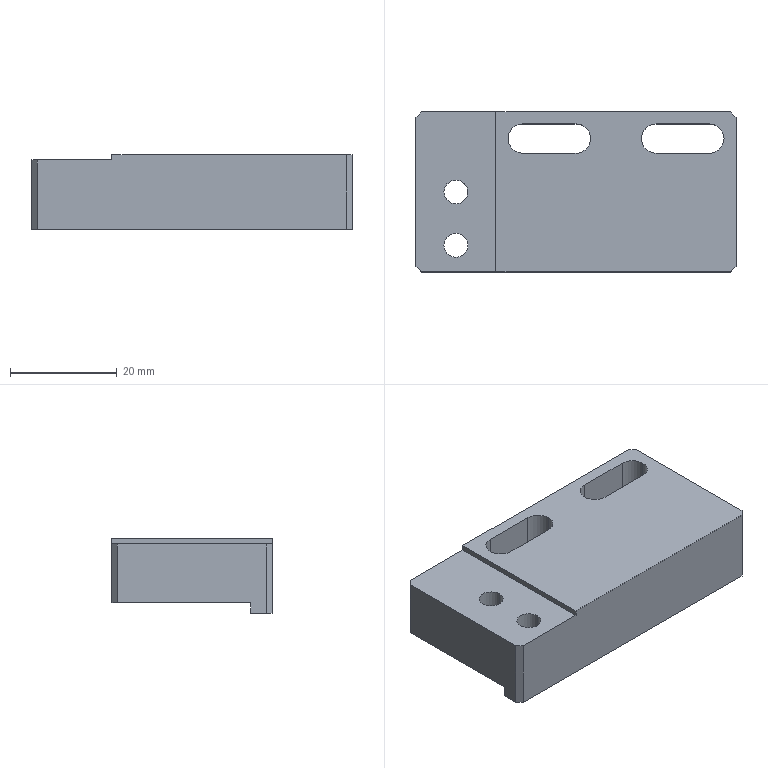Part | NX | features BREP 1 | 1 solid | 35 faces | box 60 x 30 x 14 mm | volume 19021 mm3 | plane 21 | cylinder 14 | commonest cylinder face diameters 5.5 x6 4.5 x4 8 x4
STEP:
#1=CARTESIAN_POINT('',(25.,12.75,-6.));
#2=VERTEX_POINT('',#1);
#3=CARTESIAN_POINT('',(27.75,10.,-6.));
#4=VERTEX_POINT('',#3);
#5=CARTESIAN_POINT('',(25.,10.,-6.));
#6=DIRECTION('',(0.,0.,-1.));
#7=DIRECTION('',(-1.,0.,0.));
#8=AXIS2_PLACEMENT_3D('',#5,#6,#7);
#9=CIRCLE('',#8,2.75);
#10=EDGE_CURVE('',#2,#4,#9,.T.);
#11=ORIENTED_EDGE('',*,*,#10,.T.);
#12=CARTESIAN_POINT('',(27.75,10.,6.));
#13=VERTEX_POINT('',#12);
#14=CARTESIAN_POINT('',(27.75,10.,-30.));
#15=DIRECTION('',(0.,0.,1.));
#16=VECTOR('',#15,1000.);
#17=LINE('',#14,#16);
#18=EDGE_CURVE('',#4,#13,#17,.T.);
#19=ORIENTED_EDGE('',*,*,#18,.T.);
#20=CARTESIAN_POINT('',(25.,12.75,6.));
#21=VERTEX_POINT('',#20);
#22=CARTESIAN_POINT('',(25.,10.,6.));
#23=DIRECTION('',(0.,0.,1.));
#24=DIRECTION('',(1.,0.,0.));
#25=AXIS2_PLACEMENT_3D('',#22,#23,#24);
#26=CIRCLE('',#25,2.75);
#27=EDGE_CURVE('',#13,#21,#26,.T.);
#28=ORIENTED_EDGE('',*,*,#27,.T.);
#29=CARTESIAN_POINT('',(25.,12.75,-30.));
#30=DIRECTION('',(0.,0.,1.));
#31=VECTOR('',#30,1000.);
#32=LINE('',#29,#31);
#33=EDGE_CURVE('',#2,#21,#32,.T.);
#34=ORIENTED_EDGE('',*,*,#33,.F.);
#35=EDGE_LOOP('',(#11,#19,#28,#34));
#36=FACE_BOUND('',#35,.T.);
#37=CARTESIAN_POINT('',(25.,10.,-30.));
#38=DIRECTION('',(0.,0.,1.));
#39=DIRECTION('',(1.,0.,0.));
#40=AXIS2_PLACEMENT_3D('',#37,#38,#39);
#41=CYLINDRICAL_SURFACE('',#40,2.75);
#42=ADVANCED_FACE('',(#36),#41,.F.);
#43=CARTESIAN_POINT('',(0.,12.75,-6.));
#44=VERTEX_POINT('',#43);
#45=CARTESIAN_POINT('',(2.75,10.,-6.));
#46=VERTEX_POINT('',#45);
#47=CARTESIAN_POINT('',(0.,10.,-6.));
#48=DIRECTION('',(0.,0.,-1.));
#49=DIRECTION('',(-1.,0.,0.));
#50=AXIS2_PLACEMENT_3D('',#47,#48,#49);
#51=CIRCLE('',#50,2.75);
#52=EDGE_CURVE('',#44,#46,#51,.T.);
#53=ORIENTED_EDGE('',*,*,#52,.T.);
#54=CARTESIAN_POINT('',(2.75,10.,6.));
#55=VERTEX_POINT('',#54);
#56=CARTESIAN_POINT('',(2.75,10.,-30.));
#57=DIRECTION('',(0.,0.,1.));
#58=VECTOR('',#57,1000.);
#59=LINE('',#56,#58);
#60=EDGE_CURVE('',#46,#55,#59,.T.);
#61=ORIENTED_EDGE('',*,*,#60,.T.);
#62=CARTESIAN_POINT('',(0.,12.75,6.));
#63=VERTEX_POINT('',#62);
#64=CARTESIAN_POINT('',(0.,10.,6.));
#65=DIRECTION('',(0.,0.,1.));
#66=DIRECTION('',(1.,0.,0.));
#67=AXIS2_PLACEMENT_3D('',#64,#65,#66);
#68=CIRCLE('',#67,2.75);
#69=EDGE_CURVE('',#55,#63,#68,.T.);
#70=ORIENTED_EDGE('',*,*,#69,.T.);
#71=CARTESIAN_POINT('',(0.,12.75,-30.));
#72=DIRECTION('',(0.,0.,1.));
#73=VECTOR('',#72,1000.);
#74=LINE('',#71,#73);
#75=EDGE_CURVE('',#44,#63,#74,.T.);
#76=ORIENTED_EDGE('',*,*,#75,.F.);
#77=EDGE_LOOP('',(#53,#61,#70,#76));
#78=FACE_BOUND('',#77,.T.);
#79=CARTESIAN_POINT('',(0.,10.,-30.));
#80=DIRECTION('',(0.,0.,1.));
#81=DIRECTION('',(1.,0.,0.));
#82=AXIS2_PLACEMENT_3D('',#79,#80,#81);
#83=CYLINDRICAL_SURFACE('',#82,2.75);
#84=ADVANCED_FACE('',(#78),#83,.F.);
#85=CARTESIAN_POINT('',(-18.5,0.,-1.5));
#86=VERTEX_POINT('',#85);
#87=CARTESIAN_POINT('',(-26.5,0.,-1.5));
#88=VERTEX_POINT('',#87);
#89=CARTESIAN_POINT('',(-22.5,0.,-1.5));
#90=DIRECTION('',(0.,0.,-1.));
#91=DIRECTION('',(-1.,0.,0.));
#92=AXIS2_PLACEMENT_3D('',#89,#90,#91);
#93=CIRCLE('',#92,4.);
#94=EDGE_CURVE('',#86,#88,#93,.T.);
#95=ORIENTED_EDGE('',*,*,#94,.F.);
#96=CARTESIAN_POINT('',(-18.5,0.,-6.));
#97=VERTEX_POINT('',#96);
#98=CARTESIAN_POINT('',(-18.5,0.,-6.));
#99=DIRECTION('',(0.,0.,-1.));
#100=VECTOR('',#99,1000.);
#101=LINE('',#98,#100);
#102=EDGE_CURVE('',#86,#97,#101,.T.);
#103=ORIENTED_EDGE('',*,*,#102,.T.);
#104=CARTESIAN_POINT('',(-26.5,0.,-6.));
#105=VERTEX_POINT('',#104);
#106=CARTESIAN_POINT('',(-22.5,0.,-6.));
#107=DIRECTION('',(0.,0.,-1.));
#108=DIRECTION('',(-1.,0.,0.));
#109=AXIS2_PLACEMENT_3D('',#106,#107,#108);
#110=CIRCLE('',#109,4.);
#111=EDGE_CURVE('',#97,#105,#110,.T.);
#112=ORIENTED_EDGE('',*,*,#111,.T.);
#113=CARTESIAN_POINT('',(-26.5,0.,-6.));
#114=DIRECTION('',(0.,0.,-1.));
#115=VECTOR('',#114,1000.);
#116=LINE('',#113,#115);
#117=EDGE_CURVE('',#88,#105,#116,.T.);
#118=ORIENTED_EDGE('',*,*,#117,.F.);
#119=EDGE_LOOP('',(#95,#103,#112,#118));
#120=FACE_BOUND('',#119,.T.);
#121=CARTESIAN_POINT('',(-22.5,0.,-6.));
#122=DIRECTION('',(0.,0.,-1.));
#123=DIRECTION('',(-1.,0.,0.));
#124=AXIS2_PLACEMENT_3D('',#121,#122,#123);
#125=CYLINDRICAL_SURFACE('',#124,4.);
#126=ADVANCED_FACE('',(#120),#125,.F.);
#127=CARTESIAN_POINT('',(-24.75,0.,5.));
#128=VERTEX_POINT('',#127);
#129=CARTESIAN_POINT('',(-20.25,0.,5.));
#130=VERTEX_POINT('',#129);
#131=CARTESIAN_POINT('',(-22.5,0.,5.));
#132=DIRECTION('',(0.,0.,1.));
#133=DIRECTION('',(-1.,0.,0.));
#134=AXIS2_PLACEMENT_3D('',#131,#132,#133);
#135=CIRCLE('',#134,2.25);
#136=EDGE_CURVE('',#128,#130,#135,.T.);
#137=ORIENTED_EDGE('',*,*,#136,.T.);
#138=CARTESIAN_POINT('',(-20.25,0.,-1.5));
#139=VERTEX_POINT('',#138);
#140=CARTESIAN_POINT('',(-20.25,0.,-6.));
#141=DIRECTION('',(0.,0.,-1.));
#142=VECTOR('',#141,1000.);
#143=LINE('',#140,#142);
#144=EDGE_CURVE('',#130,#139,#143,.T.);
#145=ORIENTED_EDGE('',*,*,#144,.T.);
#146=CARTESIAN_POINT('',(-24.75,0.,-1.5));
#147=VERTEX_POINT('',#146);
#148=CARTESIAN_POINT('',(-22.5,0.,-1.5));
#149=DIRECTION('',(0.,0.,-1.));
#150=DIRECTION('',(-1.,0.,0.));
#151=AXIS2_PLACEMENT_3D('',#148,#149,#150);
#152=CIRCLE('',#151,2.25);
#153=EDGE_CURVE('',#139,#147,#152,.T.);
#154=ORIENTED_EDGE('',*,*,#153,.T.);
#155=CARTESIAN_POINT('',(-24.75,0.,-6.));
#156=DIRECTION('',(0.,0.,-1.));
#157=VECTOR('',#156,1000.);
#158=LINE('',#155,#157);
#159=EDGE_CURVE('',#128,#147,#158,.T.);
#160=ORIENTED_EDGE('',*,*,#159,.F.);
#161=EDGE_LOOP('',(#137,#145,#154,#160));
#162=FACE_BOUND('',#161,.T.);
#163=CARTESIAN_POINT('',(-22.5,0.,-6.));
#164=DIRECTION('',(0.,0.,-1.));
#165=DIRECTION('',(-1.,0.,0.));
#166=AXIS2_PLACEMENT_3D('',#163,#164,#165);
#167=CYLINDRICAL_SURFACE('',#166,2.25);
#168=ADVANCED_FACE('',(#162),#167,.F.);
#169=CARTESIAN_POINT('',(-18.5,-10.,-1.5));
#170=VERTEX_POINT('',#169);
#171=CARTESIAN_POINT('',(-26.5,-10.,-1.5));
#172=VERTEX_POINT('',#171);
#173=CARTESIAN_POINT('',(-22.5,-10.,-1.5));
#174=DIRECTION('',(0.,0.,-1.));
#175=DIRECTION('',(-1.,0.,0.));
#176=AXIS2_PLACEMENT_3D('',#173,#174,#175);
#177=CIRCLE('',#176,4.);
#178=EDGE_CURVE('',#170,#172,#177,.T.);
#179=ORIENTED_EDGE('',*,*,#178,.F.);
#180=CARTESIAN_POINT('',(-18.5,-10.,-6.));
#181=VERTEX_POINT('',#180);
#182=CARTESIAN_POINT('',(-18.5,-10.,-6.));
#183=DIRECTION('',(0.,0.,-1.));
#184=VECTOR('',#183,1000.);
#185=LINE('',#182,#184);
#186=EDGE_CURVE('',#170,#181,#185,.T.);
#187=ORIENTED_EDGE('',*,*,#186,.T.);
#188=CARTESIAN_POINT('',(-18.627,-11.,-6.));
#189=VERTEX_POINT('',#188);
#190=CARTESIAN_POINT('',(-22.5,-10.,-6.));
#191=DIRECTION('',(0.,0.,-1.));
#192=DIRECTION('',(-1.,0.,0.));
#193=AXIS2_PLACEMENT_3D('',#190,#191,#192);
#194=CIRCLE('',#193,4.);
#195=EDGE_CURVE('',#181,#189,#194,.T.);
#196=ORIENTED_EDGE('',*,*,#195,.T.);
#197=CARTESIAN_POINT('',(-18.627,-11.,-8.));
#198=VERTEX_POINT('',#197);
#199=CARTESIAN_POINT('',(-18.627,-11.,-6.));
#200=DIRECTION('',(0.,0.,1.));
#201=VECTOR('',#200,1000.);
#202=LINE('',#199,#201);
#203=EDGE_CURVE('',#198,#189,#202,.T.);
#204=ORIENTED_EDGE('',*,*,#203,.F.);
#205=CARTESIAN_POINT('',(-26.373,-11.,-8.));
#206=VERTEX_POINT('',#205);
#207=CARTESIAN_POINT('',(-22.5,-10.,-8.));
#208=DIRECTION('',(0.,0.,-1.));
#209=DIRECTION('',(-1.,0.,0.));
#210=AXIS2_PLACEMENT_3D('',#207,#208,#209);
#211=CIRCLE('',#210,4.);
#212=EDGE_CURVE('',#198,#206,#211,.T.);
#213=ORIENTED_EDGE('',*,*,#212,.T.);
#214=CARTESIAN_POINT('',(-26.373,-11.,-6.));
#215=VERTEX_POINT('',#214);
#216=CARTESIAN_POINT('',(-26.373,-11.,-6.));
#217=DIRECTION('',(0.,0.,-1.));
#218=VECTOR('',#217,1000.);
#219=LINE('',#216,#218);
#220=EDGE_CURVE('',#215,#206,#219,.T.);
#221=ORIENTED_EDGE('',*,*,#220,.F.);
#222=CARTESIAN_POINT('',(-26.5,-10.,-6.));
#223=VERTEX_POINT('',#222);
#224=CARTESIAN_POINT('',(-22.5,-10.,-6.));
#225=DIRECTION('',(0.,0.,-1.));
#226=DIRECTION('',(-1.,0.,0.));
#227=AXIS2_PLACEMENT_3D('',#224,#225,#226);
#228=CIRCLE('',#227,4.);
#229=EDGE_CURVE('',#215,#223,#228,.T.);
#230=ORIENTED_EDGE('',*,*,#229,.T.);
#231=CARTESIAN_POINT('',(-26.5,-10.,-6.));
#232=DIRECTION('',(0.,0.,-1.));
#233=VECTOR('',#232,1000.);
#234=LINE('',#231,#233);
#235=EDGE_CURVE('',#172,#223,#234,.T.);
#236=ORIENTED_EDGE('',*,*,#235,.F.);
#237=EDGE_LOOP('',(#179,#187,#196,#204,#213,#221,#230,#236));
#238=FACE_BOUND('',#237,.T.);
#239=CARTESIAN_POINT('',(-22.5,-10.,-6.));
#240=DIRECTION('',(0.,0.,-1.));
#241=DIRECTION('',(-1.,0.,0.));
#242=AXIS2_PLACEMENT_3D('',#239,#240,#241);
#243=CYLINDRICAL_SURFACE('',#242,4.);
#244=ADVANCED_FACE('',(#238),#243,.F.);
#245=CARTESIAN_POINT('',(-24.75,-10.,5.));
#246=VERTEX_POINT('',#245);
#247=CARTESIAN_POINT('',(-20.25,-10.,5.));
#248=VERTEX_POINT('',#247);
#249=CARTESIAN_POINT('',(-22.5,-10.,5.));
#250=DIRECTION('',(0.,0.,1.));
#251=DIRECTION('',(-1.,0.,0.));
#252=AXIS2_PLACEMENT_3D('',#249,#250,#251);
#253=CIRCLE('',#252,2.25);
#254=EDGE_CURVE('',#246,#248,#253,.T.);
#255=ORIENTED_EDGE('',*,*,#254,.T.);
#256=CARTESIAN_POINT('',(-20.25,-10.,-1.5));
#257=VERTEX_POINT('',#256);
#258=CARTESIAN_POINT('',(-20.25,-10.,-6.));
#259=DIRECTION('',(0.,0.,-1.));
#260=VECTOR('',#259,1000.);
#261=LINE('',#258,#260);
#262=EDGE_CURVE('',#248,#257,#261,.T.);
#263=ORIENTED_EDGE('',*,*,#262,.T.);
#264=CARTESIAN_POINT('',(-24.75,-10.,-1.5));
#265=VERTEX_POINT('',#264);
#266=CARTESIAN_POINT('',(-22.5,-10.,-1.5));
#267=DIRECTION('',(0.,0.,-1.));
#268=DIRECTION('',(-1.,0.,0.));
#269=AXIS2_PLACEMENT_3D('',#266,#267,#268);
#270=CIRCLE('',#269,2.25);
#271=EDGE_CURVE('',#257,#265,#270,.T.);
#272=ORIENTED_EDGE('',*,*,#271,.T.);
#273=CARTESIAN_POINT('',(-24.75,-10.,-6.));
#274=DIRECTION('',(0.,0.,-1.));
#275=VECTOR('',#274,1000.);
#276=LINE('',#273,#275);
#277=EDGE_CURVE('',#246,#265,#276,.T.);
#278=ORIENTED_EDGE('',*,*,#277,.F.);
#279=EDGE_LOOP('',(#255,#263,#272,#278));
#280=FACE_BOUND('',#279,.T.);
#281=CARTESIAN_POINT('',(-22.5,-10.,-6.));
#282=DIRECTION('',(0.,0.,-1.));
#283=DIRECTION('',(-1.,0.,0.));
#284=AXIS2_PLACEMENT_3D('',#281,#282,#283);
#285=CYLINDRICAL_SURFACE('',#284,2.25);
#286=ADVANCED_FACE('',(#280),#285,.F.);
#287=CARTESIAN_POINT('',(-30.,-11.,-6.));
#288=VERTEX_POINT('',#287);
#289=CARTESIAN_POINT('',(30.,-11.,-6.));
#290=DIRECTION('',(1.,0.,0.));
#291=VECTOR('',#290,1000.);
#292=LINE('',#289,#291);
#293=EDGE_CURVE('',#288,#215,#292,.T.);
#294=ORIENTED_EDGE('',*,*,#293,.T.);
#295=ORIENTED_EDGE('',*,*,#220,.T.);
#296=CARTESIAN_POINT('',(-30.,-11.,-8.));
#297=VERTEX_POINT('',#296);
#298=CARTESIAN_POINT('',(30.,-11.,-8.));
#299=DIRECTION('',(1.,0.,0.));
#300=VECTOR('',#299,1000.);
#301=LINE('',#298,#300);
#302=EDGE_CURVE('',#297,#206,#301,.T.);
#303=ORIENTED_EDGE('',*,*,#302,.F.);
#304=CARTESIAN_POINT('',(-30.,-11.,-8.));
#305=DIRECTION('',(0.,0.,1.));
#306=VECTOR('',#305,1000.);
#307=LINE('',#304,#306);
#308=EDGE_CURVE('',#297,#288,#307,.T.);
#309=ORIENTED_EDGE('',*,*,#308,.T.);
#310=EDGE_LOOP('',(#294,#295,#303,#309));
#311=FACE_BOUND('',#310,.T.);
#312=CARTESIAN_POINT('',(30.,-11.,-8.));
#313=DIRECTION('',(0.,-1.,0.));
#314=DIRECTION('',(0.,0.,-1.));
#315=AXIS2_PLACEMENT_3D('',#312,#313,#314);
#316=PLANE('',#315);
#317=ADVANCED_FACE('',(#311),#316,.F.);
#318=CARTESIAN_POINT('',(30.,-14.,6.));
#319=VERTEX_POINT('',#318);
#320=CARTESIAN_POINT('',(30.,14.,6.));
#321=VERTEX_POINT('',#320);
#322=CARTESIAN_POINT('',(30.,-15.,6.));
#323=DIRECTION('',(0.,1.,0.));
#324=VECTOR('',#323,1000.);
#325=LINE('',#322,#324);
#326=EDGE_CURVE('',#319,#321,#325,.T.);
#327=ORIENTED_EDGE('',*,*,#326,.F.);
#328=CARTESIAN_POINT('',(30.,-14.,-8.));
#329=VERTEX_POINT('',#328);
#330=CARTESIAN_POINT('',(30.,-14.,6.));
#331=DIRECTION('',(0.,0.,-1.));
#332=VECTOR('',#331,1000.);
#333=LINE('',#330,#332);
#334=EDGE_CURVE('',#319,#329,#333,.T.);
#335=ORIENTED_EDGE('',*,*,#334,.T.);
#336=CARTESIAN_POINT('',(30.,-11.,-8.));
#337=VERTEX_POINT('',#336);
#338=CARTESIAN_POINT('',(30.,-14.,-8.));
#339=DIRECTION('',(0.,-1.,0.));
#340=VECTOR('',#339,1000.);
#341=LINE('',#338,#340);
#342=EDGE_CURVE('',#337,#329,#341,.T.);
#343=ORIENTED_EDGE('',*,*,#342,.F.);
#344=CARTESIAN_POINT('',(30.,-11.,-6.));
#345=VERTEX_POINT('',#344);
#346=CARTESIAN_POINT('',(30.,-11.,-8.));
#347=DIRECTION('',(0.,0.,1.));
#348=VECTOR('',#347,1000.);
#349=LINE('',#346,#348);
#350=EDGE_CURVE('',#337,#345,#349,.T.);
#351=ORIENTED_EDGE('',*,*,#350,.T.);
#352=CARTESIAN_POINT('',(30.,14.,-6.));
#353=VERTEX_POINT('',#352);
#354=CARTESIAN_POINT('',(30.,-15.,-6.));
#355=DIRECTION('',(0.,1.,0.));
#356=VECTOR('',#355,1000.);
#357=LINE('',#354,#356);
#358=EDGE_CURVE('',#345,#353,#357,.T.);
#359=ORIENTED_EDGE('',*,*,#358,.T.);
#360=CARTESIAN_POINT('',(30.,14.,6.));
#361=DIRECTION('',(0.,0.,1.));
#362=VECTOR('',#361,1000.);
#363=LINE('',#360,#362);
#364=EDGE_CURVE('',#353,#321,#363,.T.);
#365=ORIENTED_EDGE('',*,*,#364,.T.);
#366=EDGE_LOOP('',(#327,#335,#343,#351,#359,#365));
#367=FACE_BOUND('',#366,.T.);
#368=CARTESIAN_POINT('',(30.,-15.,6.));
#369=DIRECTION('',(-1.,0.,0.));
#370=DIRECTION('',(0.,0.,1.));
#371=AXIS2_PLACEMENT_3D('',#368,#369,#370);
#372=PLANE('',#371);
#373=ADVANCED_FACE('',(#367),#372,.F.);
#374=CARTESIAN_POINT('',(29.,15.,6.));
#375=VERTEX_POINT('',#374);
#376=CARTESIAN_POINT('',(-15.,15.,6.));
#377=VERTEX_POINT('',#376);
#378=CARTESIAN_POINT('',(-30.,15.,6.));
#379=DIRECTION('',(-1.,0.,0.));
#380=VECTOR('',#379,1000.);
#381=LINE('',#378,#380);
#382=EDGE_CURVE('',#375,#377,#381,.T.);
#383=ORIENTED_EDGE('',*,*,#382,.F.);
#384=CARTESIAN_POINT('',(29.,15.,-6.));
#385=VERTEX_POINT('',#384);
#386=CARTESIAN_POINT('',(29.,15.,6.));
#387=DIRECTION('',(0.,0.,-1.));
#388=VECTOR('',#387,1000.);
#389=LINE('',#386,#388);
#390=EDGE_CURVE('',#375,#385,#389,.T.);
#391=ORIENTED_EDGE('',*,*,#390,.T.);
#392=CARTESIAN_POINT('',(-29.,15.,-6.));
#393=VERTEX_POINT('',#392);
#394=CARTESIAN_POINT('',(-30.,15.,-6.));
#395=DIRECTION('',(-1.,0.,0.));
#396=VECTOR('',#395,1000.);
#397=LINE('',#394,#396);
#398=EDGE_CURVE('',#385,#393,#397,.T.);
#399=ORIENTED_EDGE('',*,*,#398,.T.);
#400=CARTESIAN_POINT('',(-29.,15.,5.));
#401=VERTEX_POINT('',#400);
#402=CARTESIAN_POINT('',(-29.,15.,6.));
#403=DIRECTION('',(0.,0.,1.));
#404=VECTOR('',#403,1000.);
#405=LINE('',#402,#404);
#406=EDGE_CURVE('',#393,#401,#405,.T.);
#407=ORIENTED_EDGE('',*,*,#406,.T.);
#408=CARTESIAN_POINT('',(-15.,15.,5.));
#409=VERTEX_POINT('',#408);
#410=CARTESIAN_POINT('',(-15.,15.,5.));
#411=DIRECTION('',(-1.,0.,0.));
#412=VECTOR('',#411,1000.);
#413=LINE('',#410,#412);
#414=EDGE_CURVE('',#409,#401,#413,.T.);
#415=ORIENTED_EDGE('',*,*,#414,.F.);
#416=CARTESIAN_POINT('',(-15.,15.,6.));
#417=DIRECTION('',(0.,0.,-1.));
#418=VECTOR('',#417,1000.);
#419=LINE('',#416,#418);
#420=EDGE_CURVE('',#377,#409,#419,.T.);
#421=ORIENTED_EDGE('',*,*,#420,.F.);
#422=EDGE_LOOP('',(#383,#391,#399,#407,#415,#421));
#423=FACE_BOUND('',#422,.T.);
#424=CARTESIAN_POINT('',(-30.,15.,6.));
#425=DIRECTION('',(0.,-1.,0.));
#426=DIRECTION('',(0.,0.,-1.));
#427=AXIS2_PLACEMENT_3D('',#424,#425,#426);
#428=PLANE('',#427);
#429=ADVANCED_FACE('',(#423),#428,.F.);
#430=CARTESIAN_POINT('',(-30.,14.,-6.));
#431=VERTEX_POINT('',#430);
#432=CARTESIAN_POINT('',(-30.,-15.,-6.));
#433=DIRECTION('',(0.,-1.,0.));
#434=VECTOR('',#433,1000.);
#435=LINE('',#432,#434);
#436=EDGE_CURVE('',#431,#288,#435,.T.);
#437=ORIENTED_EDGE('',*,*,#436,.T.);
#438=ORIENTED_EDGE('',*,*,#308,.F.);
#439=CARTESIAN_POINT('',(-30.,-14.,-8.));
#440=VERTEX_POINT('',#439);
#441=CARTESIAN_POINT('',(-30.,-11.,-8.));
#442=DIRECTION('',(0.,1.,0.));
#443=VECTOR('',#442,1000.);
#444=LINE('',#441,#443);
#445=EDGE_CURVE('',#440,#297,#444,.T.);
#446=ORIENTED_EDGE('',*,*,#445,.F.);
#447=CARTESIAN_POINT('',(-30.,-14.,5.));
#448=VERTEX_POINT('',#447);
#449=CARTESIAN_POINT('',(-30.,-14.,6.));
#450=DIRECTION('',(0.,0.,1.));
#451=VECTOR('',#450,1000.);
#452=LINE('',#449,#451);
#453=EDGE_CURVE('',#440,#448,#452,.T.);
#454=ORIENTED_EDGE('',*,*,#453,.T.);
#455=CARTESIAN_POINT('',(-30.,14.,5.));
#456=VERTEX_POINT('',#455);
#457=CARTESIAN_POINT('',(-30.,-21.,5.));
#458=DIRECTION('',(0.,1.,0.));
#459=VECTOR('',#458,1000.);
#460=LINE('',#457,#459);
#461=EDGE_CURVE('',#448,#456,#460,.T.);
#462=ORIENTED_EDGE('',*,*,#461,.T.);
#463=CARTESIAN_POINT('',(-30.,14.,6.));
#464=DIRECTION('',(0.,0.,-1.));
#465=VECTOR('',#464,1000.);
#466=LINE('',#463,#465);
#467=EDGE_CURVE('',#456,#431,#466,.T.);
#468=ORIENTED_EDGE('',*,*,#467,.T.);
#469=EDGE_LOOP('',(#437,#438,#446,#454,#462,#468));
#470=FACE_BOUND('',#469,.T.);
#471=CARTESIAN_POINT('',(-30.,-15.,6.));
#472=DIRECTION('',(1.,0.,0.));
#473=DIRECTION('',(0.,1.,0.));
#474=AXIS2_PLACEMENT_3D('',#471,#472,#473);
#475=PLANE('',#474);
#476=ADVANCED_FACE('',(#470),#475,.F.);
#477=CARTESIAN_POINT('',(-29.,-15.,5.));
#478=VERTEX_POINT('',#477);
#479=CARTESIAN_POINT('',(-29.,-15.,-8.));
#480=VERTEX_POINT('',#479);
#481=CARTESIAN_POINT('',(-29.,-15.,6.));
#482=DIRECTION('',(0.,0.,-1.));
#483=VECTOR('',#482,1000.);
#484=LINE('',#481,#483);
#485=EDGE_CURVE('',#478,#480,#484,.T.);
#486=ORIENTED_EDGE('',*,*,#485,.T.);
#487=CARTESIAN_POINT('',(29.,-15.,-8.));
#488=VERTEX_POINT('',#487);
#489=CARTESIAN_POINT('',(-29.,-15.,-8.));
#490=DIRECTION('',(-1.,0.,0.));
#491=VECTOR('',#490,1000.);
#492=LINE('',#489,#491);
#493=EDGE_CURVE('',#488,#480,#492,.T.);
#494=ORIENTED_EDGE('',*,*,#493,.F.);
#495=CARTESIAN_POINT('',(29.,-15.,6.));
#496=VERTEX_POINT('',#495);
#497=CARTESIAN_POINT('',(29.,-15.,6.));
#498=DIRECTION('',(0.,0.,1.));
#499=VECTOR('',#498,1000.);
#500=LINE('',#497,#499);
#501=EDGE_CURVE('',#488,#496,#500,.T.);
#502=ORIENTED_EDGE('',*,*,#501,.T.);
#503=CARTESIAN_POINT('',(-15.,-15.,6.));
#504=VERTEX_POINT('',#503);
#505=CARTESIAN_POINT('',(-30.,-15.,6.));
#506=DIRECTION('',(1.,0.,0.));
#507=VECTOR('',#506,1000.);
#508=LINE('',#505,#507);
#509=EDGE_CURVE('',#504,#496,#508,.T.);
#510=ORIENTED_EDGE('',*,*,#509,.F.);
#511=CARTESIAN_POINT('',(-15.,-15.,5.));
#512=VERTEX_POINT('',#511);
#513=CARTESIAN_POINT('',(-15.,-15.,6.));
#514=DIRECTION('',(0.,0.,-1.));
#515=VECTOR('',#514,1000.);
#516=LINE('',#513,#515);
#517=EDGE_CURVE('',#504,#512,#516,.T.);
#518=ORIENTED_EDGE('',*,*,#517,.T.);
#519=CARTESIAN_POINT('',(-30.,-15.,5.));
#520=DIRECTION('',(-1.,0.,0.));
#521=VECTOR('',#520,1000.);
#522=LINE('',#519,#521);
#523=EDGE_CURVE('',#512,#478,#522,.T.);
#524=ORIENTED_EDGE('',*,*,#523,.T.);
#525=EDGE_LOOP('',(#486,#494,#502,#510,#518,#524));
#526=FACE_BOUND('',#525,.T.);
#527=CARTESIAN_POINT('',(-30.,-15.,6.));
#528=DIRECTION('',(0.,1.,0.));
#529=DIRECTION('',(1.,0.,0.));
#530=AXIS2_PLACEMENT_3D('',#527,#528,#529);
#531=PLANE('',#530);
#532=ADVANCED_FACE('',(#526),#531,.F.);
#533=ORIENTED_EDGE('',*,*,#509,.T.);
#534=CARTESIAN_POINT('',(30.,-14.,6.));
#535=DIRECTION('',(0.7071,0.7071,0.));
#536=VECTOR('',#535,1000.);
#537=LINE('',#534,#536);
#538=EDGE_CURVE('',#496,#319,#537,.T.);
#539=ORIENTED_EDGE('',*,*,#538,.T.);
#540=ORIENTED_EDGE('',*,*,#326,.T.);
#541=CARTESIAN_POINT('',(29.,15.,6.));
#542=DIRECTION('',(-0.7071,0.7071,0.));
#543=VECTOR('',#542,1000.);
#544=LINE('',#541,#543);
#545=EDGE_CURVE('',#321,#375,#544,.T.);
#546=ORIENTED_EDGE('',*,*,#545,.T.);
#547=ORIENTED_EDGE('',*,*,#382,.T.);
#548=CARTESIAN_POINT('',(-15.,-21.,6.));
#549=DIRECTION('',(0.,1.,0.));
#550=VECTOR('',#549,1000.);
#551=LINE('',#548,#550);
#552=EDGE_CURVE('',#504,#377,#551,.T.);
#553=ORIENTED_EDGE('',*,*,#552,.F.);
#554=EDGE_LOOP('',(#533,#539,#540,#546,#547,#553));
#555=FACE_BOUND('',#554,.T.);
#556=CARTESIAN_POINT('',(15.,7.25,6.));
#557=VERTEX_POINT('',#556);
#558=CARTESIAN_POINT('',(25.,7.25,6.));
#559=VERTEX_POINT('',#558);
#560=CARTESIAN_POINT('',(15.,7.25,6.));
#561=DIRECTION('',(1.,0.,0.));
#562=VECTOR('',#561,1000.);
#563=LINE('',#560,#562);
#564=EDGE_CURVE('',#557,#559,#563,.T.);
#565=ORIENTED_EDGE('',*,*,#564,.F.);
#566=CARTESIAN_POINT('',(15.,12.75,6.));
#567=VERTEX_POINT('',#566);
#568=CARTESIAN_POINT('',(15.,10.,6.));
#569=DIRECTION('',(0.,0.,1.));
#570=DIRECTION('',(1.,0.,0.));
#571=AXIS2_PLACEMENT_3D('',#568,#569,#570);
#572=CIRCLE('',#571,2.75);
#573=EDGE_CURVE('',#567,#557,#572,.T.);
#574=ORIENTED_EDGE('',*,*,#573,.F.);
#575=CARTESIAN_POINT('',(15.,12.75,6.));
#576=DIRECTION('',(-1.,0.,0.));
#577=VECTOR('',#576,1000.);
#578=LINE('',#575,#577);
#579=EDGE_CURVE('',#21,#567,#578,.T.);
#580=ORIENTED_EDGE('',*,*,#579,.F.);
#581=ORIENTED_EDGE('',*,*,#27,.F.);
#582=CARTESIAN_POINT('',(25.,10.,6.));
#583=DIRECTION('',(0.,0.,1.));
#584=DIRECTION('',(1.,0.,0.));
#585=AXIS2_PLACEMENT_3D('',#582,#583,#584);
#586=CIRCLE('',#585,2.75);
#587=EDGE_CURVE('',#559,#13,#586,.T.);
#588=ORIENTED_EDGE('',*,*,#587,.F.);
#589=EDGE_LOOP('',(#565,#574,#580,#581,#588));
#590=FACE_BOUND('',#589,.T.);
#591=CARTESIAN_POINT('',(-10.,7.25,6.));
#592=VERTEX_POINT('',#591);
#593=CARTESIAN_POINT('',(0.,7.25,6.));
#594=VERTEX_POINT('',#593);
#595=CARTESIAN_POINT('',(-10.,7.25,6.));
#596=DIRECTION('',(1.,0.,0.));
#597=VECTOR('',#596,1000.);
#598=LINE('',#595,#597);
#599=EDGE_CURVE('',#592,#594,#598,.T.);
#600=ORIENTED_EDGE('',*,*,#599,.F.);
#601=CARTESIAN_POINT('',(-10.,12.75,6.));
#602=VERTEX_POINT('',#601);
#603=CARTESIAN_POINT('',(-10.,10.,6.));
#604=DIRECTION('',(0.,0.,1.));
#605=DIRECTION('',(1.,0.,0.));
#606=AXIS2_PLACEMENT_3D('',#603,#604,#605);
#607=CIRCLE('',#606,2.75);
#608=EDGE_CURVE('',#602,#592,#607,.T.);
#609=ORIENTED_EDGE('',*,*,#608,.F.);
#610=CARTESIAN_POINT('',(-10.,12.75,6.));
#611=DIRECTION('',(-1.,0.,0.));
#612=VECTOR('',#611,1000.);
#613=LINE('',#610,#612);
#614=EDGE_CURVE('',#63,#602,#613,.T.);
#615=ORIENTED_EDGE('',*,*,#614,.F.);
#616=ORIENTED_EDGE('',*,*,#69,.F.);
#617=CARTESIAN_POINT('',(0.,10.,6.));
#618=DIRECTION('',(0.,0.,1.));
#619=DIRECTION('',(1.,0.,0.));
#620=AXIS2_PLACEMENT_3D('',#617,#618,#619);
#621=CIRCLE('',#620,2.75);
#622=EDGE_CURVE('',#594,#55,#621,.T.);
#623=ORIENTED_EDGE('',*,*,#622,.F.);
#624=EDGE_LOOP('',(#600,#609,#615,#616,#623));
#625=FACE_BOUND('',#624,.T.);
#626=CARTESIAN_POINT('',(0.,0.,6.));
#627=DIRECTION('',(0.,0.,-1.));
#628=DIRECTION('',(0.,-1.,0.));
#629=AXIS2_PLACEMENT_3D('',#626,#627,#628);
#630=PLANE('',#629);
#631=ADVANCED_FACE('',(#555,#590,#625),#630,.F.);
#632=ORIENTED_EDGE('',*,*,#293,.F.);
#633=ORIENTED_EDGE('',*,*,#436,.F.);
#634=CARTESIAN_POINT('',(-22.,22.,-6.));
#635=DIRECTION('',(0.7071,0.7071,0.));
#636=VECTOR('',#635,1000.);
#637=LINE('',#634,#636);
#638=EDGE_CURVE('',#431,#393,#637,.T.);
#639=ORIENTED_EDGE('',*,*,#638,.T.);
#640=ORIENTED_EDGE('',*,*,#398,.F.);
#641=CARTESIAN_POINT('',(22.,22.,-6.));
#642=DIRECTION('',(0.7071,-0.7071,0.));
#643=VECTOR('',#642,1000.);
#644=LINE('',#641,#643);
#645=EDGE_CURVE('',#385,#353,#644,.T.);
#646=ORIENTED_EDGE('',*,*,#645,.T.);
#647=ORIENTED_EDGE('',*,*,#358,.F.);
#648=CARTESIAN_POINT('',(30.,-11.,-6.));
#649=DIRECTION('',(1.,0.,0.));
#650=VECTOR('',#649,1000.);
#651=LINE('',#648,#650);
#652=EDGE_CURVE('',#189,#345,#651,.T.);
#653=ORIENTED_EDGE('',*,*,#652,.F.);
#654=ORIENTED_EDGE('',*,*,#195,.F.);
#655=CARTESIAN_POINT('',(-22.5,-10.,-6.));
#656=DIRECTION('',(0.,0.,-1.));
#657=DIRECTION('',(-1.,0.,0.));
#658=AXIS2_PLACEMENT_3D('',#655,#656,#657);
#659=CIRCLE('',#658,4.);
#660=EDGE_CURVE('',#223,#181,#659,.T.);
#661=ORIENTED_EDGE('',*,*,#660,.F.);
#662=ORIENTED_EDGE('',*,*,#229,.F.);
#663=EDGE_LOOP('',(#632,#633,#639,#640,#646,#647,#653,#654,#661,#662));
#664=FACE_BOUND('',#663,.T.);
#665=CARTESIAN_POINT('',(15.,7.25,-6.));
#666=VERTEX_POINT('',#665);
#667=CARTESIAN_POINT('',(15.,12.75,-6.));
#668=VERTEX_POINT('',#667);
#669=CARTESIAN_POINT('',(15.,10.,-6.));
#670=DIRECTION('',(0.,0.,-1.));
#671=DIRECTION('',(-1.,0.,0.));
#672=AXIS2_PLACEMENT_3D('',#669,#670,#671);
#673=CIRCLE('',#672,2.75);
#674=EDGE_CURVE('',#666,#668,#673,.T.);
#675=ORIENTED_EDGE('',*,*,#674,.F.);
#676=CARTESIAN_POINT('',(25.,7.25,-6.));
#677=VERTEX_POINT('',#676);
#678=CARTESIAN_POINT('',(0.,7.25,-6.));
#679=DIRECTION('',(-1.,0.,0.));
#680=VECTOR('',#679,1000.);
#681=LINE('',#678,#680);
#682=EDGE_CURVE('',#677,#666,#681,.T.);
#683=ORIENTED_EDGE('',*,*,#682,.F.);
#684=CARTESIAN_POINT('',(25.,10.,-6.));
#685=DIRECTION('',(0.,0.,-1.));
#686=DIRECTION('',(-1.,0.,0.));
#687=AXIS2_PLACEMENT_3D('',#684,#685,#686);
#688=CIRCLE('',#687,2.75);
#689=EDGE_CURVE('',#4,#677,#688,.T.);
#690=ORIENTED_EDGE('',*,*,#689,.F.);
#691=ORIENTED_EDGE('',*,*,#10,.F.);
#692=CARTESIAN_POINT('',(0.,12.75,-6.));
#693=DIRECTION('',(1.,0.,0.));
#694=VECTOR('',#693,1000.);
#695=LINE('',#692,#694);
#696=EDGE_CURVE('',#668,#2,#695,.T.);
#697=ORIENTED_EDGE('',*,*,#696,.F.);
#698=EDGE_LOOP('',(#675,#683,#690,#691,#697));
#699=FACE_BOUND('',#698,.T.);
#700=CARTESIAN_POINT('',(-10.,7.25,-6.));
#701=VERTEX_POINT('',#700);
#702=CARTESIAN_POINT('',(-10.,12.75,-6.));
#703=VERTEX_POINT('',#702);
#704=CARTESIAN_POINT('',(-10.,10.,-6.));
#705=DIRECTION('',(0.,0.,-1.));
#706=DIRECTION('',(-1.,0.,0.));
#707=AXIS2_PLACEMENT_3D('',#704,#705,#706);
#708=CIRCLE('',#707,2.75);
#709=EDGE_CURVE('',#701,#703,#708,.T.);
#710=ORIENTED_EDGE('',*,*,#709,.F.);
#711=CARTESIAN_POINT('',(0.,7.25,-6.));
#712=VERTEX_POINT('',#711);
#713=CARTESIAN_POINT('',(0.,7.25,-6.));
#714=DIRECTION('',(-1.,0.,0.));
#715=VECTOR('',#714,1000.);
#716=LINE('',#713,#715);
#717=EDGE_CURVE('',#712,#701,#716,.T.);
#718=ORIENTED_EDGE('',*,*,#717,.F.);
#719=CARTESIAN_POINT('',(0.,10.,-6.));
#720=DIRECTION('',(0.,0.,-1.));
#721=DIRECTION('',(-1.,0.,0.));
#722=AXIS2_PLACEMENT_3D('',#719,#720,#721);
#723=CIRCLE('',#722,2.75);
#724=EDGE_CURVE('',#46,#712,#723,.T.);
#725=ORIENTED_EDGE('',*,*,#724,.F.);
#726=ORIENTED_EDGE('',*,*,#52,.F.);
#727=CARTESIAN_POINT('',(0.,12.75,-6.));
#728=DIRECTION('',(1.,0.,0.));
#729=VECTOR('',#728,1000.);
#730=LINE('',#727,#729);
#731=EDGE_CURVE('',#703,#44,#730,.T.);
#732=ORIENTED_EDGE('',*,*,#731,.F.);
#733=EDGE_LOOP('',(#710,#718,#725,#726,#732));
#734=FACE_BOUND('',#733,.T.);
#735=CARTESIAN_POINT('',(-22.5,0.,-6.));
#736=DIRECTION('',(0.,0.,-1.));
#737=DIRECTION('',(-1.,0.,0.));
#738=AXIS2_PLACEMENT_3D('',#735,#736,#737);
#739=CIRCLE('',#738,4.);
#740=EDGE_CURVE('',#105,#97,#739,.T.);
#741=ORIENTED_EDGE('',*,*,#740,.F.);
#742=ORIENTED_EDGE('',*,*,#111,.F.);
#743=EDGE_LOOP('',(#741,#742));
#744=FACE_BOUND('',#743,.T.);
#745=CARTESIAN_POINT('',(0.,0.,-6.));
#746=DIRECTION('',(0.,0.,-1.));
#747=DIRECTION('',(0.,-1.,0.));
#748=AXIS2_PLACEMENT_3D('',#745,#746,#747);
#749=PLANE('',#748);
#750=ADVANCED_FACE('',(#664,#699,#734,#744),#749,.T.);
#751=ORIENTED_EDGE('',*,*,#262,.F.);
#752=CARTESIAN_POINT('',(-22.5,-10.,5.));
#753=DIRECTION('',(0.,0.,1.));
#754=DIRECTION('',(-1.,0.,0.));
#755=AXIS2_PLACEMENT_3D('',#752,#753,#754);
#756=CIRCLE('',#755,2.25);
#757=EDGE_CURVE('',#248,#246,#756,.T.);
#758=ORIENTED_EDGE('',*,*,#757,.T.);
#759=ORIENTED_EDGE('',*,*,#277,.T.);
#760=CARTESIAN_POINT('',(-22.5,-10.,-1.5));
#761=DIRECTION('',(0.,0.,-1.));
#762=DIRECTION('',(-1.,0.,0.));
#763=AXIS2_PLACEMENT_3D('',#760,#761,#762);
#764=CIRCLE('',#763,2.25);
#765=EDGE_CURVE('',#265,#257,#764,.T.);
#766=ORIENTED_EDGE('',*,*,#765,.T.);
#767=EDGE_LOOP('',(#751,#758,#759,#766));
#768=FACE_BOUND('',#767,.T.);
#769=CARTESIAN_POINT('',(-22.5,-10.,-6.));
#770=DIRECTION('',(0.,0.,-1.));
#771=DIRECTION('',(-1.,0.,0.));
#772=AXIS2_PLACEMENT_3D('',#769,#770,#771);
#773=CYLINDRICAL_SURFACE('',#772,2.25);
#774=ADVANCED_FACE('',(#768),#773,.F.);
#775=CARTESIAN_POINT('',(-22.5,-10.,-1.5));
#776=DIRECTION('',(0.,0.,-1.));
#777=DIRECTION('',(-1.,0.,0.));
#778=AXIS2_PLACEMENT_3D('',#775,#776,#777);
#779=CIRCLE('',#778,4.);
#780=EDGE_CURVE('',#172,#170,#779,.T.);
#781=ORIENTED_EDGE('',*,*,#780,.T.);
#782=ORIENTED_EDGE('',*,*,#178,.T.);
#783=EDGE_LOOP('',(#781,#782));
#784=FACE_BOUND('',#783,.T.);
#785=ORIENTED_EDGE('',*,*,#765,.F.);
#786=ORIENTED_EDGE('',*,*,#271,.F.);
#787=EDGE_LOOP('',(#785,#786));
#788=FACE_BOUND('',#787,.T.);
#789=CARTESIAN_POINT('',(-20.25,-10.,-1.5));
#790=DIRECTION('',(0.,0.,1.));
#791=DIRECTION('',(1.,0.,0.));
#792=AXIS2_PLACEMENT_3D('',#789,#790,#791);
#793=PLANE('',#792);
#794=ADVANCED_FACE('',(#784,#788),#793,.F.);
#795=ORIENTED_EDGE('',*,*,#186,.F.);
#796=ORIENTED_EDGE('',*,*,#780,.F.);
#797=ORIENTED_EDGE('',*,*,#235,.T.);
#798=ORIENTED_EDGE('',*,*,#660,.T.);
#799=EDGE_LOOP('',(#795,#796,#797,#798));
#800=FACE_BOUND('',#799,.T.);
#801=CARTESIAN_POINT('',(-22.5,-10.,-6.));
#802=DIRECTION('',(0.,0.,-1.));
#803=DIRECTION('',(-1.,0.,0.));
#804=AXIS2_PLACEMENT_3D('',#801,#802,#803);
#805=CYLINDRICAL_SURFACE('',#804,4.);
#806=ADVANCED_FACE('',(#800),#805,.F.);
#807=ORIENTED_EDGE('',*,*,#144,.F.);
#808=CARTESIAN_POINT('',(-22.5,0.,5.));
#809=DIRECTION('',(0.,0.,1.));
#810=DIRECTION('',(-1.,0.,0.));
#811=AXIS2_PLACEMENT_3D('',#808,#809,#810);
#812=CIRCLE('',#811,2.25);
#813=EDGE_CURVE('',#130,#128,#812,.T.);
#814=ORIENTED_EDGE('',*,*,#813,.T.);
#815=ORIENTED_EDGE('',*,*,#159,.T.);
#816=CARTESIAN_POINT('',(-22.5,0.,-1.5));
#817=DIRECTION('',(0.,0.,-1.));
#818=DIRECTION('',(-1.,0.,0.));
#819=AXIS2_PLACEMENT_3D('',#816,#817,#818);
#820=CIRCLE('',#819,2.25);
#821=EDGE_CURVE('',#147,#139,#820,.T.);
#822=ORIENTED_EDGE('',*,*,#821,.T.);
#823=EDGE_LOOP('',(#807,#814,#815,#822));
#824=FACE_BOUND('',#823,.T.);
#825=CARTESIAN_POINT('',(-22.5,0.,-6.));
#826=DIRECTION('',(0.,0.,-1.));
#827=DIRECTION('',(-1.,0.,0.));
#828=AXIS2_PLACEMENT_3D('',#825,#826,#827);
#829=CYLINDRICAL_SURFACE('',#828,2.25);
#830=ADVANCED_FACE('',(#824),#829,.F.);
#831=CARTESIAN_POINT('',(-22.5,0.,-1.5));
#832=DIRECTION('',(0.,0.,-1.));
#833=DIRECTION('',(-1.,0.,0.));
#834=AXIS2_PLACEMENT_3D('',#831,#832,#833);
#835=CIRCLE('',#834,4.);
#836=EDGE_CURVE('',#88,#86,#835,.T.);
#837=ORIENTED_EDGE('',*,*,#836,.T.);
#838=ORIENTED_EDGE('',*,*,#94,.T.);
#839=EDGE_LOOP('',(#837,#838));
#840=FACE_BOUND('',#839,.T.);
#841=ORIENTED_EDGE('',*,*,#821,.F.);
#842=ORIENTED_EDGE('',*,*,#153,.F.);
#843=EDGE_LOOP('',(#841,#842));
#844=FACE_BOUND('',#843,.T.);
#845=CARTESIAN_POINT('',(-20.25,0.,-1.5));
#846=DIRECTION('',(0.,0.,1.));
#847=DIRECTION('',(1.,0.,0.));
#848=AXIS2_PLACEMENT_3D('',#845,#846,#847);
#849=PLANE('',#848);
#850=ADVANCED_FACE('',(#840,#844),#849,.F.);
#851=ORIENTED_EDGE('',*,*,#102,.F.);
#852=ORIENTED_EDGE('',*,*,#836,.F.);
#853=ORIENTED_EDGE('',*,*,#117,.T.);
#854=ORIENTED_EDGE('',*,*,#740,.T.);
#855=EDGE_LOOP('',(#851,#852,#853,#854));
#856=FACE_BOUND('',#855,.T.);
#857=CARTESIAN_POINT('',(-22.5,0.,-6.));
#858=DIRECTION('',(0.,0.,-1.));
#859=DIRECTION('',(-1.,0.,0.));
#860=AXIS2_PLACEMENT_3D('',#857,#858,#859);
#861=CYLINDRICAL_SURFACE('',#860,4.);
#862=ADVANCED_FACE('',(#856),#861,.F.);
#863=ORIENTED_EDGE('',*,*,#552,.T.);
#864=ORIENTED_EDGE('',*,*,#420,.T.);
#865=CARTESIAN_POINT('',(-15.,-21.,5.));
#866=DIRECTION('',(0.,1.,0.));
#867=VECTOR('',#866,1000.);
#868=LINE('',#865,#867);
#869=EDGE_CURVE('',#512,#409,#868,.T.);
#870=ORIENTED_EDGE('',*,*,#869,.F.);
#871=ORIENTED_EDGE('',*,*,#517,.F.);
#872=EDGE_LOOP('',(#863,#864,#870,#871));
#873=FACE_BOUND('',#872,.T.);
#874=CARTESIAN_POINT('',(-15.,-21.,6.));
#875=DIRECTION('',(1.,0.,0.));
#876=DIRECTION('',(0.,1.,0.));
#877=AXIS2_PLACEMENT_3D('',#874,#875,#876);
#878=PLANE('',#877);
#879=ADVANCED_FACE('',(#873),#878,.F.);
#880=ORIENTED_EDGE('',*,*,#461,.F.);
#881=CARTESIAN_POINT('',(-29.,-15.,5.));
#882=DIRECTION('',(0.7071,-0.7071,0.));
#883=VECTOR('',#882,1000.);
#884=LINE('',#881,#883);
#885=EDGE_CURVE('',#448,#478,#884,.T.);
#886=ORIENTED_EDGE('',*,*,#885,.T.);
#887=ORIENTED_EDGE('',*,*,#523,.F.);
#888=ORIENTED_EDGE('',*,*,#869,.T.);
#889=ORIENTED_EDGE('',*,*,#414,.T.);
#890=CARTESIAN_POINT('',(-30.,14.,5.));
#891=DIRECTION('',(-0.7071,-0.7071,0.));
#892=VECTOR('',#891,1000.);
#893=LINE('',#890,#892);
#894=EDGE_CURVE('',#401,#456,#893,.T.);
#895=ORIENTED_EDGE('',*,*,#894,.T.);
#896=EDGE_LOOP('',(#880,#886,#887,#888,#889,#895));
#897=FACE_BOUND('',#896,.T.);
#898=ORIENTED_EDGE('',*,*,#254,.F.);
#899=ORIENTED_EDGE('',*,*,#757,.F.);
#900=EDGE_LOOP('',(#898,#899));
#901=FACE_BOUND('',#900,.T.);
#902=ORIENTED_EDGE('',*,*,#136,.F.);
#903=ORIENTED_EDGE('',*,*,#813,.F.);
#904=EDGE_LOOP('',(#902,#903));
#905=FACE_BOUND('',#904,.T.);
#906=CARTESIAN_POINT('',(-15.,-21.,5.));
#907=DIRECTION('',(0.,0.,-1.));
#908=DIRECTION('',(-1.,0.,0.));
#909=AXIS2_PLACEMENT_3D('',#906,#907,#908);
#910=PLANE('',#909);
#911=ADVANCED_FACE('',(#897,#901,#905),#910,.F.);
#912=ORIENTED_EDGE('',*,*,#709,.T.);
#913=CARTESIAN_POINT('',(-10.,12.75,-30.));
#914=DIRECTION('',(0.,0.,1.));
#915=VECTOR('',#914,1000.);
#916=LINE('',#913,#915);
#917=EDGE_CURVE('',#703,#602,#916,.T.);
#918=ORIENTED_EDGE('',*,*,#917,.T.);
#919=ORIENTED_EDGE('',*,*,#608,.T.);
#920=CARTESIAN_POINT('',(-10.,7.25,-30.));
#921=DIRECTION('',(0.,0.,1.));
#922=VECTOR('',#921,1000.);
#923=LINE('',#920,#922);
#924=EDGE_CURVE('',#701,#592,#923,.T.);
#925=ORIENTED_EDGE('',*,*,#924,.F.);
#926=EDGE_LOOP('',(#912,#918,#919,#925));
#927=FACE_BOUND('',#926,.T.);
#928=CARTESIAN_POINT('',(-10.,10.,-30.));
#929=DIRECTION('',(0.,0.,1.));
#930=DIRECTION('',(1.,0.,0.));
#931=AXIS2_PLACEMENT_3D('',#928,#929,#930);
#932=CYLINDRICAL_SURFACE('',#931,2.75);
#933=ADVANCED_FACE('',(#927),#932,.F.);
#934=ORIENTED_EDGE('',*,*,#731,.T.);
#935=ORIENTED_EDGE('',*,*,#75,.T.);
#936=ORIENTED_EDGE('',*,*,#614,.T.);
#937=ORIENTED_EDGE('',*,*,#917,.F.);
#938=EDGE_LOOP('',(#934,#935,#936,#937));
#939=FACE_BOUND('',#938,.T.);
#940=CARTESIAN_POINT('',(-10.,12.75,-30.));
#941=DIRECTION('',(0.,1.,0.));
#942=DIRECTION('',(1.,0.,0.));
#943=AXIS2_PLACEMENT_3D('',#940,#941,#942);
#944=PLANE('',#943);
#945=ADVANCED_FACE('',(#939),#944,.F.);
#946=ORIENTED_EDGE('',*,*,#60,.F.);
#947=ORIENTED_EDGE('',*,*,#724,.T.);
#948=CARTESIAN_POINT('',(0.,7.25,-30.));
#949=DIRECTION('',(0.,0.,1.));
#950=VECTOR('',#949,1000.);
#951=LINE('',#948,#950);
#952=EDGE_CURVE('',#712,#594,#951,.T.);
#953=ORIENTED_EDGE('',*,*,#952,.T.);
#954=ORIENTED_EDGE('',*,*,#622,.T.);
#955=EDGE_LOOP('',(#946,#947,#953,#954));
#956=FACE_BOUND('',#955,.T.);
#957=CARTESIAN_POINT('',(0.,10.,-30.));
#958=DIRECTION('',(0.,0.,1.));
#959=DIRECTION('',(1.,0.,0.));
#960=AXIS2_PLACEMENT_3D('',#957,#958,#959);
#961=CYLINDRICAL_SURFACE('',#960,2.75);
#962=ADVANCED_FACE('',(#956),#961,.F.);
#963=ORIENTED_EDGE('',*,*,#717,.T.);
#964=ORIENTED_EDGE('',*,*,#924,.T.);
#965=ORIENTED_EDGE('',*,*,#599,.T.);
#966=ORIENTED_EDGE('',*,*,#952,.F.);
#967=EDGE_LOOP('',(#963,#964,#965,#966));
#968=FACE_BOUND('',#967,.T.);
#969=CARTESIAN_POINT('',(-10.,7.25,-30.));
#970=DIRECTION('',(0.,-1.,0.));
#971=DIRECTION('',(0.,0.,-1.));
#972=AXIS2_PLACEMENT_3D('',#969,#970,#971);
#973=PLANE('',#972);
#974=ADVANCED_FACE('',(#968),#973,.F.);
#975=ORIENTED_EDGE('',*,*,#674,.T.);
#976=CARTESIAN_POINT('',(15.,12.75,-30.));
#977=DIRECTION('',(0.,0.,1.));
#978=VECTOR('',#977,1000.);
#979=LINE('',#976,#978);
#980=EDGE_CURVE('',#668,#567,#979,.T.);
#981=ORIENTED_EDGE('',*,*,#980,.T.);
#982=ORIENTED_EDGE('',*,*,#573,.T.);
#983=CARTESIAN_POINT('',(15.,7.25,-30.));
#984=DIRECTION('',(0.,0.,1.));
#985=VECTOR('',#984,1000.);
#986=LINE('',#983,#985);
#987=EDGE_CURVE('',#666,#557,#986,.T.);
#988=ORIENTED_EDGE('',*,*,#987,.F.);
#989=EDGE_LOOP('',(#975,#981,#982,#988));
#990=FACE_BOUND('',#989,.T.);
#991=CARTESIAN_POINT('',(15.,10.,-30.));
#992=DIRECTION('',(0.,0.,1.));
#993=DIRECTION('',(1.,0.,0.));
#994=AXIS2_PLACEMENT_3D('',#991,#992,#993);
#995=CYLINDRICAL_SURFACE('',#994,2.75);
#996=ADVANCED_FACE('',(#990),#995,.F.);
#997=ORIENTED_EDGE('',*,*,#696,.T.);
#998=ORIENTED_EDGE('',*,*,#33,.T.);
#999=ORIENTED_EDGE('',*,*,#579,.T.);
#1000=ORIENTED_EDGE('',*,*,#980,.F.);
#1001=EDGE_LOOP('',(#997,#998,#999,#1000));
#1002=FACE_BOUND('',#1001,.T.);
#1003=CARTESIAN_POINT('',(15.,12.75,-30.));
#1004=DIRECTION('',(0.,1.,0.));
#1005=DIRECTION('',(1.,0.,0.));
#1006=AXIS2_PLACEMENT_3D('',#1003,#1004,#1005);
#1007=PLANE('',#1006);
#1008=ADVANCED_FACE('',(#1002),#1007,.F.);
#1009=ORIENTED_EDGE('',*,*,#18,.F.);
#1010=ORIENTED_EDGE('',*,*,#689,.T.);
#1011=CARTESIAN_POINT('',(25.,7.25,-30.));
#1012=DIRECTION('',(0.,0.,1.));
#1013=VECTOR('',#1012,1000.);
#1014=LINE('',#1011,#1013);
#1015=EDGE_CURVE('',#677,#559,#1014,.T.);
#1016=ORIENTED_EDGE('',*,*,#1015,.T.);
#1017=ORIENTED_EDGE('',*,*,#587,.T.);
#1018=EDGE_LOOP('',(#1009,#1010,#1016,#1017));
#1019=FACE_BOUND('',#1018,.T.);
#1020=CARTESIAN_POINT('',(25.,10.,-30.));
#1021=DIRECTION('',(0.,0.,1.));
#1022=DIRECTION('',(1.,0.,0.));
#1023=AXIS2_PLACEMENT_3D('',#1020,#1021,#1022);
#1024=CYLINDRICAL_SURFACE('',#1023,2.75);
#1025=ADVANCED_FACE('',(#1019),#1024,.F.);
#1026=ORIENTED_EDGE('',*,*,#682,.T.);
#1027=ORIENTED_EDGE('',*,*,#987,.T.);
#1028=ORIENTED_EDGE('',*,*,#564,.T.);
#1029=ORIENTED_EDGE('',*,*,#1015,.F.);
#1030=EDGE_LOOP('',(#1026,#1027,#1028,#1029));
#1031=FACE_BOUND('',#1030,.T.);
#1032=CARTESIAN_POINT('',(15.,7.25,-30.));
#1033=DIRECTION('',(0.,-1.,0.));
#1034=DIRECTION('',(0.,0.,-1.));
#1035=AXIS2_PLACEMENT_3D('',#1032,#1033,#1034);
#1036=PLANE('',#1035);
#1037=ADVANCED_FACE('',(#1031),#1036,.F.);
#1038=ORIENTED_EDGE('',*,*,#538,.F.);
#1039=ORIENTED_EDGE('',*,*,#501,.F.);
#1040=CARTESIAN_POINT('',(29.,-15.,-8.));
#1041=DIRECTION('',(-0.7071,-0.7071,0.));
#1042=VECTOR('',#1041,1000.);
#1043=LINE('',#1040,#1042);
#1044=EDGE_CURVE('',#329,#488,#1043,.T.);
#1045=ORIENTED_EDGE('',*,*,#1044,.F.);
#1046=ORIENTED_EDGE('',*,*,#334,.F.);
#1047=EDGE_LOOP('',(#1038,#1039,#1045,#1046));
#1048=FACE_BOUND('',#1047,.T.);
#1049=CARTESIAN_POINT('',(30.,-14.,6.));
#1050=DIRECTION('',(-0.7071,0.7071,0.));
#1051=DIRECTION('',(0.,0.,1.));
#1052=AXIS2_PLACEMENT_3D('',#1049,#1050,#1051);
#1053=PLANE('',#1052);
#1054=ADVANCED_FACE('',(#1048),#1053,.F.);
#1055=ORIENTED_EDGE('',*,*,#545,.F.);
#1056=ORIENTED_EDGE('',*,*,#364,.F.);
#1057=ORIENTED_EDGE('',*,*,#645,.F.);
#1058=ORIENTED_EDGE('',*,*,#390,.F.);
#1059=EDGE_LOOP('',(#1055,#1056,#1057,#1058));
#1060=FACE_BOUND('',#1059,.T.);
#1061=CARTESIAN_POINT('',(29.,15.,6.));
#1062=DIRECTION('',(-0.7071,-0.7071,0.));
#1063=DIRECTION('',(-0.7071,0.7071,0.));
#1064=AXIS2_PLACEMENT_3D('',#1061,#1062,#1063);
#1065=PLANE('',#1064);
#1066=ADVANCED_FACE('',(#1060),#1065,.F.);
#1067=ORIENTED_EDGE('',*,*,#885,.F.);
#1068=ORIENTED_EDGE('',*,*,#453,.F.);
#1069=CARTESIAN_POINT('',(-29.,-15.,-8.));
#1070=DIRECTION('',(-0.7071,0.7071,0.));
#1071=VECTOR('',#1070,1000.);
#1072=LINE('',#1069,#1071);
#1073=EDGE_CURVE('',#480,#440,#1072,.T.);
#1074=ORIENTED_EDGE('',*,*,#1073,.F.);
#1075=ORIENTED_EDGE('',*,*,#485,.F.);
#1076=EDGE_LOOP('',(#1067,#1068,#1074,#1075));
#1077=FACE_BOUND('',#1076,.T.);
#1078=CARTESIAN_POINT('',(-29.,-15.,6.));
#1079=DIRECTION('',(0.7071,0.7071,0.));
#1080=DIRECTION('',(0.,0.,-1.));
#1081=AXIS2_PLACEMENT_3D('',#1078,#1079,#1080);
#1082=PLANE('',#1081);
#1083=ADVANCED_FACE('',(#1077),#1082,.F.);
#1084=ORIENTED_EDGE('',*,*,#894,.F.);
#1085=ORIENTED_EDGE('',*,*,#406,.F.);
#1086=ORIENTED_EDGE('',*,*,#638,.F.);
#1087=ORIENTED_EDGE('',*,*,#467,.F.);
#1088=EDGE_LOOP('',(#1084,#1085,#1086,#1087));
#1089=FACE_BOUND('',#1088,.T.);
#1090=CARTESIAN_POINT('',(-30.,14.,6.));
#1091=DIRECTION('',(0.7071,-0.7071,0.));
#1092=DIRECTION('',(0.,0.,-1.));
#1093=AXIS2_PLACEMENT_3D('',#1090,#1091,#1092);
#1094=PLANE('',#1093);
#1095=ADVANCED_FACE('',(#1089),#1094,.F.);
#1096=CARTESIAN_POINT('',(30.,-11.,-8.));
#1097=DIRECTION('',(1.,0.,0.));
#1098=VECTOR('',#1097,1000.);
#1099=LINE('',#1096,#1098);
#1100=EDGE_CURVE('',#198,#337,#1099,.T.);
#1101=ORIENTED_EDGE('',*,*,#1100,.F.);
#1102=ORIENTED_EDGE('',*,*,#203,.T.);
#1103=ORIENTED_EDGE('',*,*,#652,.T.);
#1104=ORIENTED_EDGE('',*,*,#350,.F.);
#1105=EDGE_LOOP('',(#1101,#1102,#1103,#1104));
#1106=FACE_BOUND('',#1105,.T.);
#1107=CARTESIAN_POINT('',(30.,-11.,-8.));
#1108=DIRECTION('',(0.,-1.,0.));
#1109=DIRECTION('',(0.,0.,-1.));
#1110=AXIS2_PLACEMENT_3D('',#1107,#1108,#1109);
#1111=PLANE('',#1110);
#1112=ADVANCED_FACE('',(#1106),#1111,.F.);
#1113=ORIENTED_EDGE('',*,*,#302,.T.);
#1114=ORIENTED_EDGE('',*,*,#212,.F.);
#1115=ORIENTED_EDGE('',*,*,#1100,.T.);
#1116=ORIENTED_EDGE('',*,*,#342,.T.);
#1117=ORIENTED_EDGE('',*,*,#1044,.T.);
#1118=ORIENTED_EDGE('',*,*,#493,.T.);
#1119=ORIENTED_EDGE('',*,*,#1073,.T.);
#1120=ORIENTED_EDGE('',*,*,#445,.T.);
#1121=EDGE_LOOP('',(#1113,#1114,#1115,#1116,#1117,#1118,#1119,#1120));
#1122=FACE_BOUND('',#1121,.T.);
#1123=CARTESIAN_POINT('',(0.,0.,-8.));
#1124=DIRECTION('',(0.,0.,1.));
#1125=DIRECTION('',(1.,0.,0.));
#1126=AXIS2_PLACEMENT_3D('',#1123,#1124,#1125);
#1127=PLANE('',#1126);
#1128=ADVANCED_FACE('',(#1122),#1127,.F.);
#1129=CLOSED_SHELL('',(#42,#84,#126,#168,#244,#286,#317,#373,#429,#476,#532,#631,#750,#774,#794,#806,#830,#850,#862,#879,#911,#933,#945,#962,#974,#996,#1008,#1025,#1037,#1054,#1066,#1083,#1095,#1112,#1128));
#1130=MANIFOLD_SOLID_BREP('',#1129);
#1131=(LENGTH_UNIT()NAMED_UNIT(*)SI_UNIT(.MILLI.,.METRE.));
#1132=UNCERTAINTY_MEASURE_WITH_UNIT(LENGTH_MEASURE(0.00001),#1131,'','');
#1133=(NAMED_UNIT(*)PLANE_ANGLE_UNIT()SI_UNIT($,.RADIAN.));
#1134=(NAMED_UNIT(*)SI_UNIT($,.STERADIAN.)SOLID_ANGLE_UNIT());
#1135=(GEOMETRIC_REPRESENTATION_CONTEXT(3)GLOBAL_UNCERTAINTY_ASSIGNED_CONTEXT((#1132))GLOBAL_UNIT_ASSIGNED_CONTEXT((#1131,#1133,#1134))REPRESENTATION_CONTEXT('',''));
#1136=ADVANCED_BREP_SHAPE_REPRESENTATION('',(#1130),#1135);